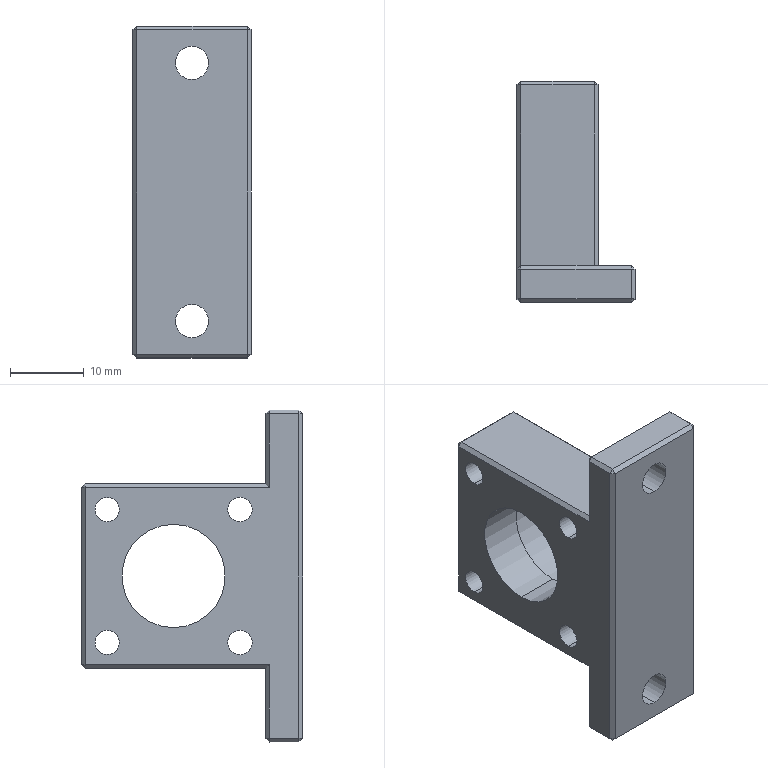Part | STEP file | 06-13 Push-pull bearing seat | 1 solid | 60 faces | box 16 x 30 x 45 mm | volume 7960 mm3 | plane 44 | cylinder 16 | commonest cylinder face diameters 3.3 x8 4.5 x4 14 x2 16 x2